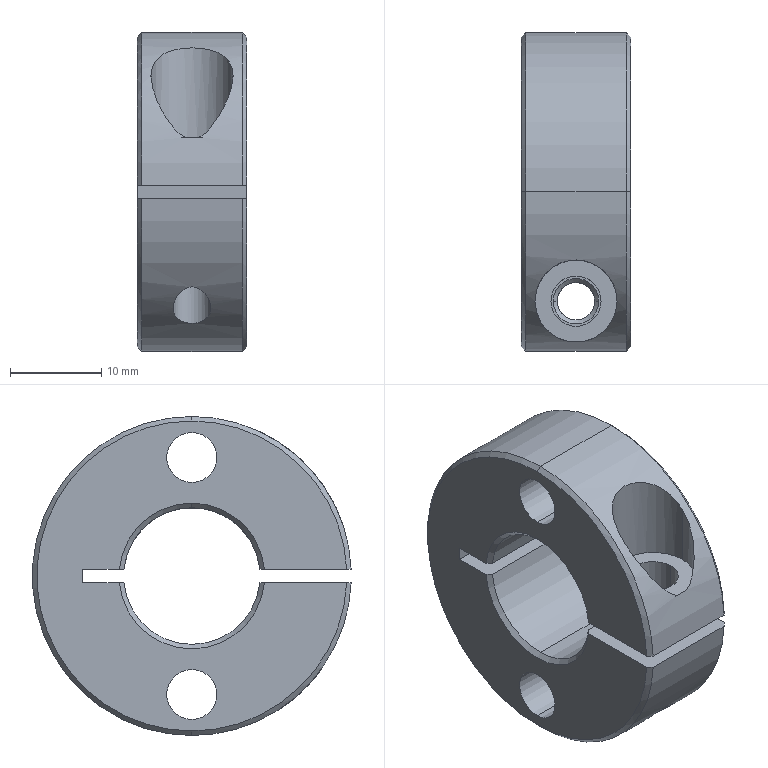Part | STEP file | 0232_Z_SSCSM15-12_1 | 1 solid | 39 faces | box 12 x 34.984 x 35 mm | volume 7867 mm3 | cylinder 17 | cone 14 | plane 8 | commonest cylinder face diameters 5.5 x6 9 x3 15 x3 35 x3 4.134 x2